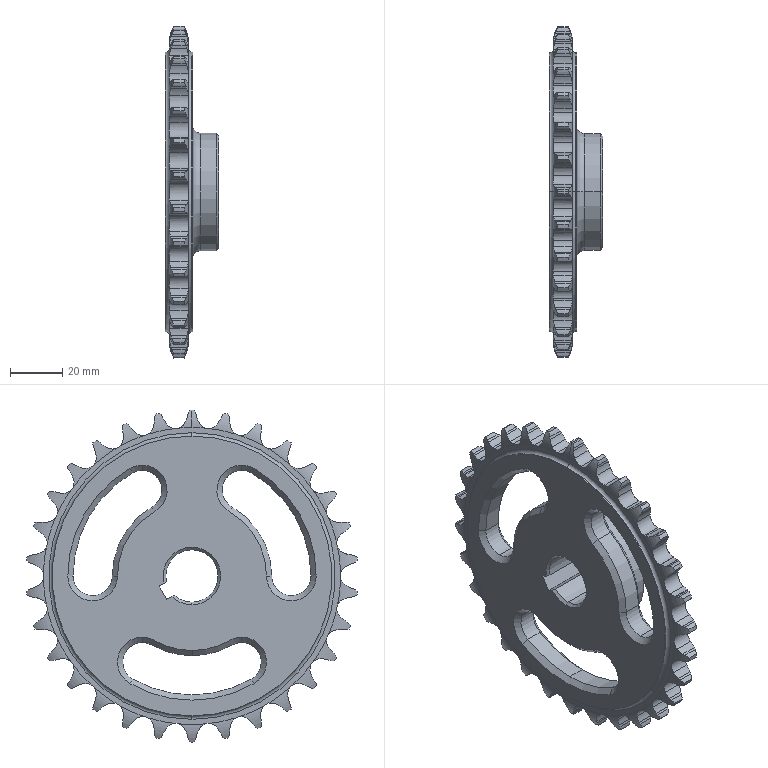Part | SolidWorks | features BaseBody 1 | 1 solid | 395 faces | box 20.59 x 126.465 x 127 mm | volume 93015 mm3 | cylinder 222 | torus 68 | plane 68 | cone 37 | commonest cylinder face diameters 11.344 x64 20.732 x64 8.06 x38 127 x31 15 x8 61 x4